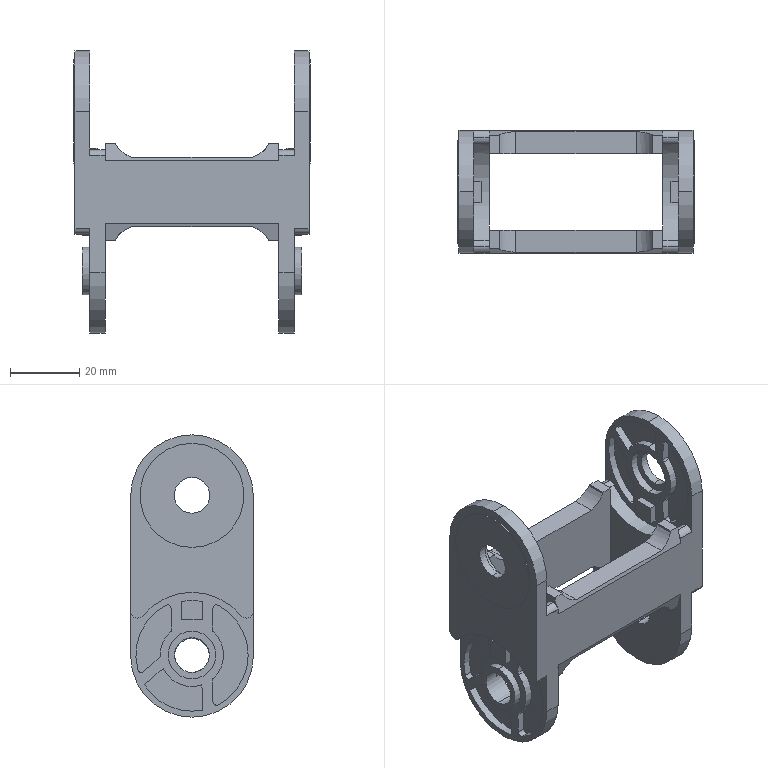Part | SolidWorks | features BaseBody 1 | 1 solid | 240 faces | box 68 x 35.356 x 81.35 mm | volume 37089 mm3 | cylinder 130 | plane 110 | commonest cylinder face diameters 2 x40 4.24 x12 10 x8 13.7 x8 15.6 x8 18.2 x8